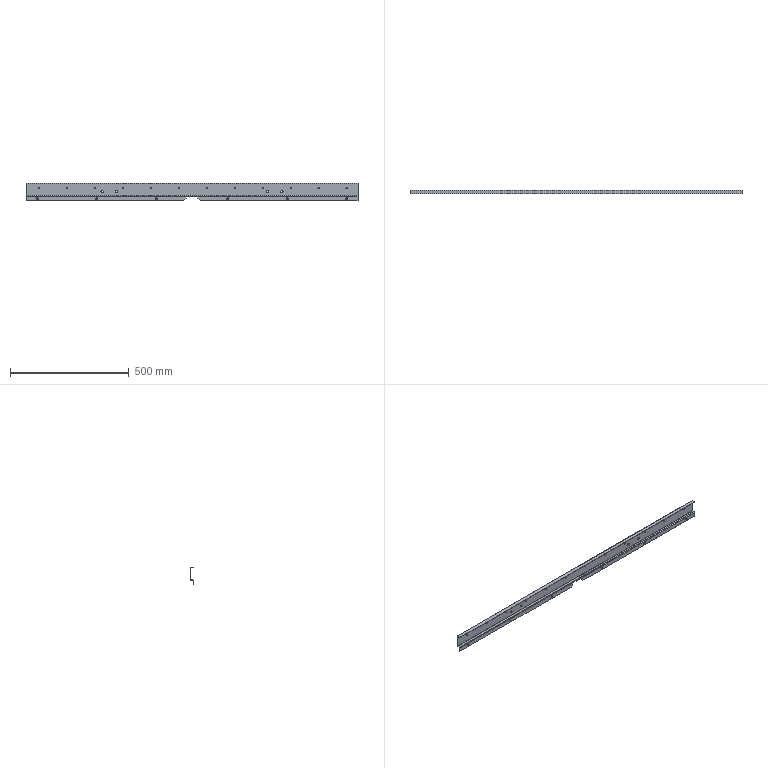Part | NX | features solid 2 | 1 solid | 70 faces | box 1395 x 16 x 73.5 mm | volume 204351 mm3 | cylinder 50 | plane 20 | commonest cylinder face diameters 6 x25 8 x12 9.2 x8 1 x2 4 x2 3 x1